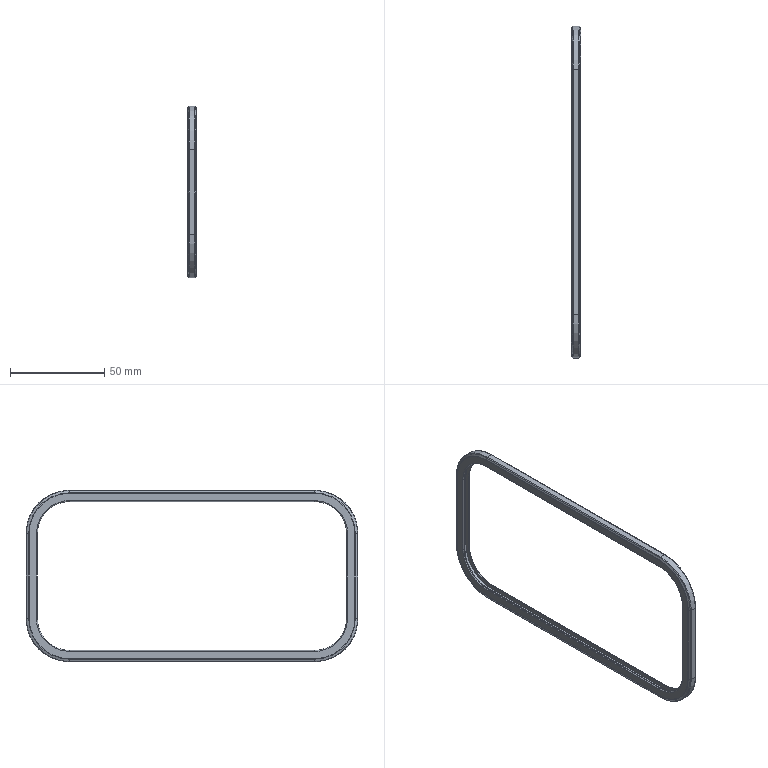Part | SolidWorks | features BaseBody 1 | 1 solid | 100 faces | box 4.9 x 176 x 91 mm | volume 10787 mm3 | cylinder 40 | plane 28 | spline 24 | cone 8 | commonest cylinder face diameters 1 x24 34 x8 38 x4 46 x4